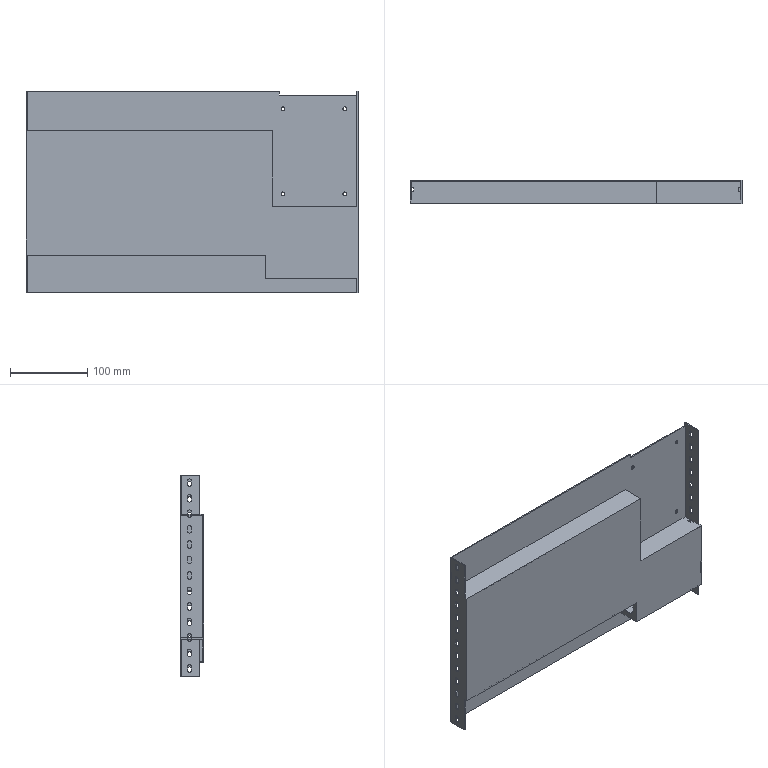Part | SolidWorks | features ICE 19, LPattern 2, Extrusion 1, Fillet 1 | 1 solid | 182 faces | box 429 x 30.5 x 260 mm | volume 225455 mm3 | plane 92 | cylinder 90 | commonest cylinder face diameters 5 x86 14 x2 20 x2